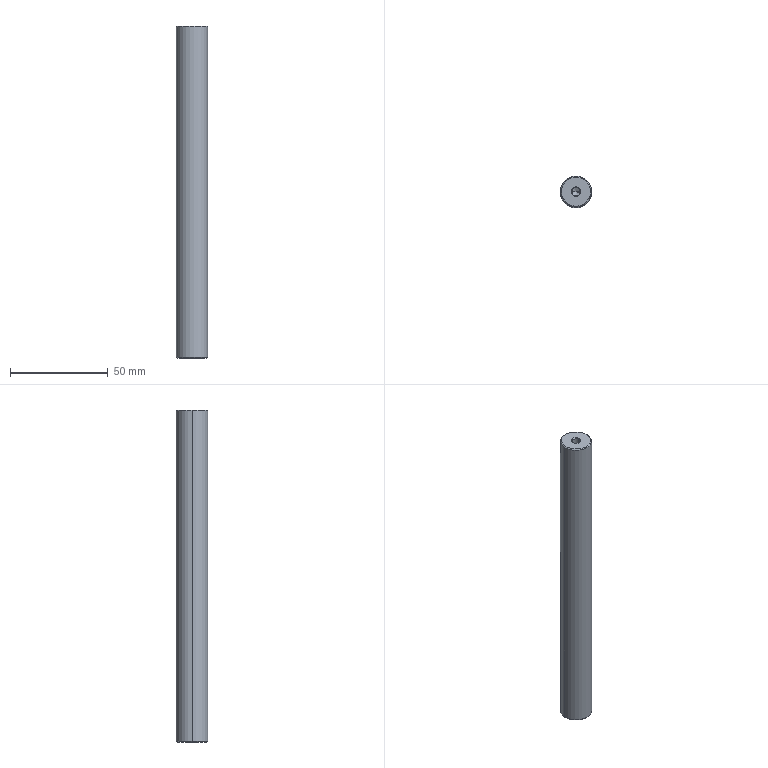Part | STEP file | 001-003-SCJ22_D16_L170_M5_N5 | 1 solid | 20 faces | box 16 x 16 x 170 mm | volume 33866 mm3 | cone 12 | cylinder 6 | plane 2 | commonest cylinder face diameters 4.134 x4 16 x2
STEP:
#1=CARTESIAN_POINT('',(0.,0.,0.));
#2=DIRECTION('',(0.,0.,1.));
#3=DIRECTION('',(1.,0.,0.));
#4=AXIS2_PLACEMENT_3D('',#1,#2,#3);
#5=CARTESIAN_POINT('',(0.,2.067,-159.25));
#6=VERTEX_POINT('',#5);
#7=CARTESIAN_POINT('',(0.,-2.067,-159.25));
#8=VERTEX_POINT('',#7);
#9=CARTESIAN_POINT('',(0.,0.,-159.25));
#10=DIRECTION('',(0.,0.,1.));
#11=DIRECTION('',(0.,-1.,0.));
#12=AXIS2_PLACEMENT_3D('',#9,#10,#11);
#13=CIRCLE('',#12,2.067);
#14=CARTESIAN_POINT('',(0.,0.,-159.25));
#15=DIRECTION('',(0.,0.,-1.));
#16=DIRECTION('',(0.,1.,0.));
#17=AXIS2_PLACEMENT_3D('',#14,#15,#16);
#18=CONICAL_SURFACE('',#17,2.067,1.047);
#19=CARTESIAN_POINT('',(9.425,0.));
#20=DIRECTION('',(-1.,0.));
#21=VECTOR('',#20,1.);
#22=LINE('',#19,#21);
#23=(GEOMETRIC_REPRESENTATION_CONTEXT(2)PARAMETRIC_REPRESENTATION_CONTEXT()REPRESENTATION_CONTEXT('',''));
#24=DEFINITIONAL_REPRESENTATION('',(#22),#23);
#25=PCURVE('',#18,#24);
#26=CARTESIAN_POINT('',(0.,0.,-170.));
#27=DIRECTION('',(0.,0.,1.));
#28=DIRECTION('',(0.,-1.,0.));
#29=AXIS2_PLACEMENT_3D('',#26,#27,#28);
#30=CYLINDRICAL_SURFACE('',#29,2.067);
#31=CARTESIAN_POINT('',(0.,10.75));
#32=DIRECTION('',(1.,0.));
#33=VECTOR('',#32,1.);
#34=LINE('',#31,#33);
#35=(GEOMETRIC_REPRESENTATION_CONTEXT(2)PARAMETRIC_REPRESENTATION_CONTEXT()REPRESENTATION_CONTEXT('',''));
#36=DEFINITIONAL_REPRESENTATION('',(#34),#35);
#37=PCURVE('',#30,#36);
#38=SURFACE_CURVE('',#13,(#25,#37),.PCURVE_S1.);
#39=EDGE_CURVE('',#6,#8,#38,.T.);
#40=ORIENTED_EDGE('',*,*,#39,.T.);
#41=CARTESIAN_POINT('',(0.,0.,-158.057));
#42=VERTEX_POINT('',#41);
#43=CARTESIAN_POINT('',(0.,-2.067,-159.25));
#44=DIRECTION('',(0.,-0.866,-0.5));
#45=VECTOR('',#44,1.);
#46=LINE('',#43,#45);
#47=CARTESIAN_POINT('',(3.142,0.));
#48=DIRECTION('',(0.,1.));
#49=VECTOR('',#48,1.);
#50=LINE('',#47,#49);
#51=(GEOMETRIC_REPRESENTATION_CONTEXT(2)PARAMETRIC_REPRESENTATION_CONTEXT()REPRESENTATION_CONTEXT('',''));
#52=DEFINITIONAL_REPRESENTATION('',(#50),#51);
#53=PCURVE('',#18,#52);
#54=CARTESIAN_POINT('',(0.,0.,-159.25));
#55=DIRECTION('',(0.,0.,-1.));
#56=DIRECTION('',(0.,1.,0.));
#57=AXIS2_PLACEMENT_3D('',#54,#55,#56);
#58=CONICAL_SURFACE('',#57,2.067,1.047);
#59=CARTESIAN_POINT('',(3.142,0.));
#60=DIRECTION('',(0.,1.));
#61=VECTOR('',#60,1.);
#62=LINE('',#59,#61);
#63=(GEOMETRIC_REPRESENTATION_CONTEXT(2)PARAMETRIC_REPRESENTATION_CONTEXT()REPRESENTATION_CONTEXT('',''));
#64=DEFINITIONAL_REPRESENTATION('',(#62),#63);
#65=PCURVE('',#58,#64);
#66=SURFACE_CURVE('',#46,(#53,#65),.PCURVE_S1.);
#67=EDGE_CURVE('',#42,#8,#66,.T.);
#68=ORIENTED_EDGE('',*,*,#67,.F.);
#69=CARTESIAN_POINT('',(0.,2.067,-159.25));
#70=DIRECTION('',(0.,0.866,-0.5));
#71=VECTOR('',#70,1.);
#72=LINE('',#69,#71);
#73=CARTESIAN_POINT('',(6.283,0.));
#74=DIRECTION('',(0.,1.));
#75=VECTOR('',#74,1.);
#76=LINE('',#73,#75);
#77=(GEOMETRIC_REPRESENTATION_CONTEXT(2)PARAMETRIC_REPRESENTATION_CONTEXT()REPRESENTATION_CONTEXT('',''));
#78=DEFINITIONAL_REPRESENTATION('',(#76),#77);
#79=PCURVE('',#18,#78);
#80=CARTESIAN_POINT('',(0.,0.));
#81=DIRECTION('',(0.,1.));
#82=VECTOR('',#81,1.);
#83=LINE('',#80,#82);
#84=(GEOMETRIC_REPRESENTATION_CONTEXT(2)PARAMETRIC_REPRESENTATION_CONTEXT()REPRESENTATION_CONTEXT('',''));
#85=DEFINITIONAL_REPRESENTATION('',(#83),#84);
#86=PCURVE('',#58,#85);
#87=SURFACE_CURVE('',#72,(#79,#86),.PCURVE_S1.);
#88=EDGE_CURVE('',#42,#6,#87,.T.);
#89=ORIENTED_EDGE('',*,*,#88,.T.);
#90=EDGE_LOOP('',(#40,#68,#89));
#91=FACE_BOUND('',#90,.F.);
#92=ADVANCED_FACE('',(#91),#18,.F.);
#93=CARTESIAN_POINT('',(0.,-2.067,-169.567));
#94=VERTEX_POINT('',#93);
#95=CARTESIAN_POINT('',(0.,-2.067,-170.));
#96=DIRECTION('',(0.,0.,1.));
#97=VECTOR('',#96,1.);
#98=LINE('',#95,#97);
#99=CARTESIAN_POINT('',(6.283,0.));
#100=DIRECTION('',(0.,1.));
#101=VECTOR('',#100,1.);
#102=LINE('',#99,#101);
#103=(GEOMETRIC_REPRESENTATION_CONTEXT(2)PARAMETRIC_REPRESENTATION_CONTEXT()REPRESENTATION_CONTEXT('',''));
#104=DEFINITIONAL_REPRESENTATION('',(#102),#103);
#105=PCURVE('',#30,#104);
#106=CARTESIAN_POINT('',(0.,0.,-170.));
#107=DIRECTION('',(0.,0.,1.));
#108=DIRECTION('',(0.,-1.,0.));
#109=AXIS2_PLACEMENT_3D('',#106,#107,#108);
#110=CYLINDRICAL_SURFACE('',#109,2.067);
#111=CARTESIAN_POINT('',(0.,0.));
#112=DIRECTION('',(0.,1.));
#113=VECTOR('',#112,1.);
#114=LINE('',#111,#113);
#115=(GEOMETRIC_REPRESENTATION_CONTEXT(2)PARAMETRIC_REPRESENTATION_CONTEXT()REPRESENTATION_CONTEXT('',''));
#116=DEFINITIONAL_REPRESENTATION('',(#114),#115);
#117=PCURVE('',#110,#116);
#118=SURFACE_CURVE('',#98,(#105,#117),.PCURVE_S1.);
#119=EDGE_CURVE('',#94,#8,#118,.T.);
#120=ORIENTED_EDGE('',*,*,#119,.T.);
#121=ORIENTED_EDGE('',*,*,#39,.F.);
#122=CARTESIAN_POINT('',(0.,2.067,-169.567));
#123=VERTEX_POINT('',#122);
#124=CARTESIAN_POINT('',(0.,2.067,-170.));
#125=DIRECTION('',(0.,0.,1.));
#126=VECTOR('',#125,1.);
#127=LINE('',#124,#126);
#128=CARTESIAN_POINT('',(3.142,0.));
#129=DIRECTION('',(0.,1.));
#130=VECTOR('',#129,1.);
#131=LINE('',#128,#130);
#132=(GEOMETRIC_REPRESENTATION_CONTEXT(2)PARAMETRIC_REPRESENTATION_CONTEXT()REPRESENTATION_CONTEXT('',''));
#133=DEFINITIONAL_REPRESENTATION('',(#131),#132);
#134=PCURVE('',#30,#133);
#135=CARTESIAN_POINT('',(3.142,0.));
#136=DIRECTION('',(0.,1.));
#137=VECTOR('',#136,1.);
#138=LINE('',#135,#137);
#139=(GEOMETRIC_REPRESENTATION_CONTEXT(2)PARAMETRIC_REPRESENTATION_CONTEXT()REPRESENTATION_CONTEXT('',''));
#140=DEFINITIONAL_REPRESENTATION('',(#138),#139);
#141=PCURVE('',#110,#140);
#142=SURFACE_CURVE('',#127,(#134,#141),.PCURVE_S1.);
#143=EDGE_CURVE('',#123,#6,#142,.T.);
#144=ORIENTED_EDGE('',*,*,#143,.F.);
#145=CARTESIAN_POINT('',(0.,0.,-169.567));
#146=DIRECTION('',(0.,0.,1.));
#147=DIRECTION('',(0.,-1.,0.));
#148=AXIS2_PLACEMENT_3D('',#145,#146,#147);
#149=CIRCLE('',#148,2.067);
#150=CARTESIAN_POINT('',(0.,0.433));
#151=DIRECTION('',(1.,0.));
#152=VECTOR('',#151,1.);
#153=LINE('',#150,#152);
#154=(GEOMETRIC_REPRESENTATION_CONTEXT(2)PARAMETRIC_REPRESENTATION_CONTEXT()REPRESENTATION_CONTEXT('',''));
#155=DEFINITIONAL_REPRESENTATION('',(#153),#154);
#156=PCURVE('',#30,#155);
#157=CARTESIAN_POINT('',(0.,0.,-170.));
#158=DIRECTION('',(0.,0.,-1.));
#159=DIRECTION('',(0.,1.,0.));
#160=AXIS2_PLACEMENT_3D('',#157,#158,#159);
#161=CONICAL_SURFACE('',#160,2.5,0.7854);
#162=CARTESIAN_POINT('',(9.425,-0.433));
#163=DIRECTION('',(-1.,0.));
#164=VECTOR('',#163,1.);
#165=LINE('',#162,#164);
#166=(GEOMETRIC_REPRESENTATION_CONTEXT(2)PARAMETRIC_REPRESENTATION_CONTEXT()REPRESENTATION_CONTEXT('',''));
#167=DEFINITIONAL_REPRESENTATION('',(#165),#166);
#168=PCURVE('',#161,#167);
#169=SURFACE_CURVE('',#149,(#156,#168),.PCURVE_S1.);
#170=EDGE_CURVE('',#123,#94,#169,.T.);
#171=ORIENTED_EDGE('',*,*,#170,.T.);
#172=EDGE_LOOP('',(#120,#121,#144,#171));
#173=FACE_BOUND('',#172,.F.);
#174=ADVANCED_FACE('',(#173),#30,.F.);
#175=CARTESIAN_POINT('',(0.,2.5,-170.));
#176=VERTEX_POINT('',#175);
#177=CARTESIAN_POINT('',(0.,2.5,-170.));
#178=DIRECTION('',(0.,0.7071,-0.7071));
#179=VECTOR('',#178,1.);
#180=LINE('',#177,#179);
#181=CARTESIAN_POINT('',(6.283,0.));
#182=DIRECTION('',(0.,1.));
#183=VECTOR('',#182,1.);
#184=LINE('',#181,#183);
#185=(GEOMETRIC_REPRESENTATION_CONTEXT(2)PARAMETRIC_REPRESENTATION_CONTEXT()REPRESENTATION_CONTEXT('',''));
#186=DEFINITIONAL_REPRESENTATION('',(#184),#185);
#187=PCURVE('',#161,#186);
#188=CARTESIAN_POINT('',(0.,0.,-170.));
#189=DIRECTION('',(0.,0.,-1.));
#190=DIRECTION('',(0.,1.,0.));
#191=AXIS2_PLACEMENT_3D('',#188,#189,#190);
#192=CONICAL_SURFACE('',#191,2.5,0.7854);
#193=CARTESIAN_POINT('',(0.,0.));
#194=DIRECTION('',(0.,1.));
#195=VECTOR('',#194,1.);
#196=LINE('',#193,#195);
#197=(GEOMETRIC_REPRESENTATION_CONTEXT(2)PARAMETRIC_REPRESENTATION_CONTEXT()REPRESENTATION_CONTEXT('',''));
#198=DEFINITIONAL_REPRESENTATION('',(#196),#197);
#199=PCURVE('',#192,#198);
#200=SURFACE_CURVE('',#180,(#187,#199),.PCURVE_S1.);
#201=EDGE_CURVE('',#123,#176,#200,.T.);
#202=ORIENTED_EDGE('',*,*,#201,.T.);
#203=CARTESIAN_POINT('',(0.,-2.5,-170.));
#204=VERTEX_POINT('',#203);
#205=CARTESIAN_POINT('',(0.,0.,-170.));
#206=DIRECTION('',(0.,0.,1.));
#207=DIRECTION('',(0.,-1.,0.));
#208=AXIS2_PLACEMENT_3D('',#205,#206,#207);
#209=CIRCLE('',#208,2.5);
#210=CARTESIAN_POINT('',(9.425,0.));
#211=DIRECTION('',(-1.,0.));
#212=VECTOR('',#211,1.);
#213=LINE('',#210,#212);
#214=(GEOMETRIC_REPRESENTATION_CONTEXT(2)PARAMETRIC_REPRESENTATION_CONTEXT()REPRESENTATION_CONTEXT('',''));
#215=DEFINITIONAL_REPRESENTATION('',(#213),#214);
#216=PCURVE('',#161,#215);
#217=CARTESIAN_POINT('',(0.,7.5,-170.));
#218=DIRECTION('',(0.,0.,1.));
#219=DIRECTION('',(1.,0.,0.));
#220=AXIS2_PLACEMENT_3D('',#217,#218,#219);
#221=PLANE('',#220);
#222=CARTESIAN_POINT('',(0.,-7.5));
#223=DIRECTION('',(0.,-1.));
#224=AXIS2_PLACEMENT_2D('',#222,#223);
#225=CIRCLE('',#224,2.5);
#226=(GEOMETRIC_REPRESENTATION_CONTEXT(2)PARAMETRIC_REPRESENTATION_CONTEXT()REPRESENTATION_CONTEXT('',''));
#227=DEFINITIONAL_REPRESENTATION('',(#225),#226);
#228=PCURVE('',#221,#227);
#229=SURFACE_CURVE('',#209,(#216,#228),.PCURVE_S1.);
#230=EDGE_CURVE('',#176,#204,#229,.T.);
#231=ORIENTED_EDGE('',*,*,#230,.T.);
#232=CARTESIAN_POINT('',(0.,-2.5,-170.));
#233=DIRECTION('',(0.,-0.7071,-0.7071));
#234=VECTOR('',#233,1.);
#235=LINE('',#232,#234);
#236=CARTESIAN_POINT('',(3.142,0.));
#237=DIRECTION('',(0.,1.));
#238=VECTOR('',#237,1.);
#239=LINE('',#236,#238);
#240=(GEOMETRIC_REPRESENTATION_CONTEXT(2)PARAMETRIC_REPRESENTATION_CONTEXT()REPRESENTATION_CONTEXT('',''));
#241=DEFINITIONAL_REPRESENTATION('',(#239),#240);
#242=PCURVE('',#161,#241);
#243=CARTESIAN_POINT('',(3.142,0.));
#244=DIRECTION('',(0.,1.));
#245=VECTOR('',#244,1.);
#246=LINE('',#243,#245);
#247=(GEOMETRIC_REPRESENTATION_CONTEXT(2)PARAMETRIC_REPRESENTATION_CONTEXT()REPRESENTATION_CONTEXT('',''));
#248=DEFINITIONAL_REPRESENTATION('',(#246),#247);
#249=PCURVE('',#192,#248);
#250=SURFACE_CURVE('',#235,(#242,#249),.PCURVE_S1.);
#251=EDGE_CURVE('',#94,#204,#250,.T.);
#252=ORIENTED_EDGE('',*,*,#251,.F.);
#253=ORIENTED_EDGE('',*,*,#170,.F.);
#254=EDGE_LOOP('',(#202,#231,#252,#253));
#255=FACE_BOUND('',#254,.F.);
#256=ADVANCED_FACE('',(#255),#161,.F.);
#257=CARTESIAN_POINT('',(-2.067,0.,-10.75));
#258=VERTEX_POINT('',#257);
#259=CARTESIAN_POINT('',(2.067,0.,-10.75));
#260=VERTEX_POINT('',#259);
#261=CARTESIAN_POINT('',(0.,0.,-10.75));
#262=DIRECTION('',(0.,0.,1.));
#263=DIRECTION('',(1.,0.,0.));
#264=AXIS2_PLACEMENT_3D('',#261,#262,#263);
#265=CIRCLE('',#264,2.067);
#266=CARTESIAN_POINT('',(0.,0.,988.057));
#267=DIRECTION('',(0.,0.,1.));
#268=DIRECTION('',(1.,0.,0.));
#269=AXIS2_PLACEMENT_3D('',#266,#267,#268);
#270=CONICAL_SURFACE('',#269,1732.051,1.047);
#271=CARTESIAN_POINT('',(0.,-998.807));
#272=DIRECTION('',(1.,0.));
#273=VECTOR('',#272,1.);
#274=LINE('',#271,#273);
#275=(GEOMETRIC_REPRESENTATION_CONTEXT(2)PARAMETRIC_REPRESENTATION_CONTEXT()REPRESENTATION_CONTEXT('',''));
#276=DEFINITIONAL_REPRESENTATION('',(#274),#275);
#277=PCURVE('',#270,#276);
#278=CARTESIAN_POINT('',(0.,0.,-11.943));
#279=DIRECTION('',(0.,0.,1.));
#280=DIRECTION('',(1.,0.,0.));
#281=AXIS2_PLACEMENT_3D('',#278,#279,#280);
#282=CYLINDRICAL_SURFACE('',#281,2.067);
#283=CARTESIAN_POINT('',(0.,1.193));
#284=DIRECTION('',(1.,0.));
#285=VECTOR('',#284,1.);
#286=LINE('',#283,#285);
#287=(GEOMETRIC_REPRESENTATION_CONTEXT(2)PARAMETRIC_REPRESENTATION_CONTEXT()REPRESENTATION_CONTEXT('',''));
#288=DEFINITIONAL_REPRESENTATION('',(#286),#287);
#289=PCURVE('',#282,#288);
#290=SURFACE_CURVE('',#265,(#277,#289),.PCURVE_S1.);
#291=EDGE_CURVE('',#258,#260,#290,.T.);
#292=ORIENTED_EDGE('',*,*,#291,.F.);
#293=CARTESIAN_POINT('',(0.,0.,-11.943));
#294=VERTEX_POINT('',#293);
#295=CARTESIAN_POINT('',(0.,0.,-11.943));
#296=DIRECTION('',(-0.866,0.,0.5));
#297=VECTOR('',#296,1.);
#298=LINE('',#295,#297);
#299=CARTESIAN_POINT('',(3.142,-1000.));
#300=CARTESIAN_POINT('',(3.142,-999.982));
#301=CARTESIAN_POINT('',(3.142,-999.946));
#302=CARTESIAN_POINT('',(3.142,-999.892));
#303=CARTESIAN_POINT('',(3.142,-999.837));
#304=CARTESIAN_POINT('',(3.142,-999.783));
#305=CARTESIAN_POINT('',(3.142,-999.729));
#306=CARTESIAN_POINT('',(3.142,-999.675));
#307=CARTESIAN_POINT('',(3.142,-999.62));
#308=CARTESIAN_POINT('',(3.142,-999.566));
#309=CARTESIAN_POINT('',(3.142,-999.512));
#310=CARTESIAN_POINT('',(3.142,-999.458));
#311=CARTESIAN_POINT('',(3.142,-999.403));
#312=CARTESIAN_POINT('',(3.142,-999.349));
#313=CARTESIAN_POINT('',(3.142,-999.295));
#314=CARTESIAN_POINT('',(3.142,-999.241));
#315=CARTESIAN_POINT('',(3.142,-999.186));
#316=CARTESIAN_POINT('',(3.142,-999.132));
#317=CARTESIAN_POINT('',(3.142,-999.078));
#318=CARTESIAN_POINT('',(3.142,-999.024));
#319=CARTESIAN_POINT('',(3.142,-998.969));
#320=CARTESIAN_POINT('',(3.142,-998.915));
#321=CARTESIAN_POINT('',(3.142,-998.861));
#322=CARTESIAN_POINT('',(3.142,-998.825));
#323=CARTESIAN_POINT('',(3.142,-998.807));
#324=B_SPLINE_CURVE_WITH_KNOTS('',3,(#299,#300,#301,#302,#303,#304,#305,#306,#307,#308,#309,#310,#311,#312,#313,#314,#315,#316,#317,#318,#319,#320,#321,#322,#323),.UNSPECIFIED.,.F.,.F.,(4,1,1,1,1,1,1,1,1,1,1,1,1,1,1,1,1,1,1,1,1,1,4),(0.,0.1085,0.217,0.3255,0.434,0.5424,0.6509,0.7594,0.8679,0.9764,1.085,1.193,1.302,1.41,1.519,1.627,1.736,1.844,1.953,2.061,2.17,2.278,2.387),.QUASI_UNIFORM_KNOTS.);
#325=(GEOMETRIC_REPRESENTATION_CONTEXT(2)PARAMETRIC_REPRESENTATION_CONTEXT()REPRESENTATION_CONTEXT('',''));
#326=DEFINITIONAL_REPRESENTATION('',(#324),#325);
#327=PCURVE('',#270,#326);
#328=CARTESIAN_POINT('',(0.,0.,988.057));
#329=DIRECTION('',(0.,0.,1.));
#330=DIRECTION('',(1.,0.,0.));
#331=AXIS2_PLACEMENT_3D('',#328,#329,#330);
#332=CONICAL_SURFACE('',#331,1732.051,1.047);
#333=CARTESIAN_POINT('',(3.142,-1000.));
#334=CARTESIAN_POINT('',(3.142,-999.982));
#335=CARTESIAN_POINT('',(3.142,-999.946));
#336=CARTESIAN_POINT('',(3.142,-999.892));
#337=CARTESIAN_POINT('',(3.142,-999.837));
#338=CARTESIAN_POINT('',(3.142,-999.783));
#339=CARTESIAN_POINT('',(3.142,-999.729));
#340=CARTESIAN_POINT('',(3.142,-999.675));
#341=CARTESIAN_POINT('',(3.142,-999.62));
#342=CARTESIAN_POINT('',(3.142,-999.566));
#343=CARTESIAN_POINT('',(3.142,-999.512));
#344=CARTESIAN_POINT('',(3.142,-999.458));
#345=CARTESIAN_POINT('',(3.142,-999.403));
#346=CARTESIAN_POINT('',(3.142,-999.349));
#347=CARTESIAN_POINT('',(3.142,-999.295));
#348=CARTESIAN_POINT('',(3.142,-999.241));
#349=CARTESIAN_POINT('',(3.142,-999.186));
#350=CARTESIAN_POINT('',(3.142,-999.132));
#351=CARTESIAN_POINT('',(3.142,-999.078));
#352=CARTESIAN_POINT('',(3.142,-999.024));
#353=CARTESIAN_POINT('',(3.142,-998.969));
#354=CARTESIAN_POINT('',(3.142,-998.915));
#355=CARTESIAN_POINT('',(3.142,-998.861));
#356=CARTESIAN_POINT('',(3.142,-998.825));
#357=CARTESIAN_POINT('',(3.142,-998.807));
#358=B_SPLINE_CURVE_WITH_KNOTS('',3,(#333,#334,#335,#336,#337,#338,#339,#340,#341,#342,#343,#344,#345,#346,#347,#348,#349,#350,#351,#352,#353,#354,#355,#356,#357),.UNSPECIFIED.,.F.,.F.,(4,1,1,1,1,1,1,1,1,1,1,1,1,1,1,1,1,1,1,1,1,1,4),(0.,0.1085,0.217,0.3255,0.434,0.5424,0.6509,0.7594,0.8679,0.9764,1.085,1.193,1.302,1.41,1.519,1.627,1.736,1.844,1.953,2.061,2.17,2.278,2.387),.QUASI_UNIFORM_KNOTS.);
#359=(GEOMETRIC_REPRESENTATION_CONTEXT(2)PARAMETRIC_REPRESENTATION_CONTEXT()REPRESENTATION_CONTEXT('',''));
#360=DEFINITIONAL_REPRESENTATION('',(#358),#359);
#361=PCURVE('',#332,#360);
#362=SURFACE_CURVE('',#298,(#327,#361),.PCURVE_S1.);
#363=EDGE_CURVE('',#294,#258,#362,.T.);
#364=ORIENTED_EDGE('',*,*,#363,.F.);
#365=CARTESIAN_POINT('',(0.,0.,-11.943));
#366=DIRECTION('',(0.866,0.,0.5));
#367=VECTOR('',#366,1.);
#368=LINE('',#365,#367);
#369=CARTESIAN_POINT('',(6.283,-1000.));
#370=DIRECTION('',(0.,1.));
#371=VECTOR('',#370,1.);
#372=LINE('',#369,#371);
#373=(GEOMETRIC_REPRESENTATION_CONTEXT(2)PARAMETRIC_REPRESENTATION_CONTEXT()REPRESENTATION_CONTEXT('',''));
#374=DEFINITIONAL_REPRESENTATION('',(#372),#373);
#375=PCURVE('',#270,#374);
#376=CARTESIAN_POINT('',(0.,-1000.));
#377=DIRECTION('',(0.,1.));
#378=VECTOR('',#377,1.);
#379=LINE('',#376,#378);
#380=(GEOMETRIC_REPRESENTATION_CONTEXT(2)PARAMETRIC_REPRESENTATION_CONTEXT()REPRESENTATION_CONTEXT('',''));
#381=DEFINITIONAL_REPRESENTATION('',(#379),#380);
#382=PCURVE('',#332,#381);
#383=SURFACE_CURVE('',#368,(#375,#382),.PCURVE_S1.);
#384=EDGE_CURVE('',#294,#260,#383,.T.);
#385=ORIENTED_EDGE('',*,*,#384,.T.);
#386=EDGE_LOOP('',(#292,#364,#385));
#387=FACE_BOUND('',#386,.F.);
#388=ADVANCED_FACE('',(#387),#270,.F.);
#389=CARTESIAN_POINT('',(2.067,0.,-0.433));
#390=VERTEX_POINT('',#389);
#391=CARTESIAN_POINT('',(2.067,0.,-11.943));
#392=DIRECTION('',(0.,0.,1.));
#393=VECTOR('',#392,1.);
#394=LINE('',#391,#393);
#395=CARTESIAN_POINT('',(6.283,0.));
#396=DIRECTION('',(0.,1.));
#397=VECTOR('',#396,1.);
#398=LINE('',#395,#397);
#399=(GEOMETRIC_REPRESENTATION_CONTEXT(2)PARAMETRIC_REPRESENTATION_CONTEXT()REPRESENTATION_CONTEXT('',''));
#400=DEFINITIONAL_REPRESENTATION('',(#398),#399);
#401=PCURVE('',#282,#400);
#402=CARTESIAN_POINT('',(0.,0.,-11.943));
#403=DIRECTION('',(0.,0.,1.));
#404=DIRECTION('',(1.,0.,0.));
#405=AXIS2_PLACEMENT_3D('',#402,#403,#404);
#406=CYLINDRICAL_SURFACE('',#405,2.067);
#407=CARTESIAN_POINT('',(0.,0.));
#408=DIRECTION('',(0.,1.));
#409=VECTOR('',#408,1.);
#410=LINE('',#407,#409);
#411=(GEOMETRIC_REPRESENTATION_CONTEXT(2)PARAMETRIC_REPRESENTATION_CONTEXT()REPRESENTATION_CONTEXT('',''));
#412=DEFINITIONAL_REPRESENTATION('',(#410),#411);
#413=PCURVE('',#406,#412);
#414=SURFACE_CURVE('',#394,(#401,#413),.PCURVE_S1.);
#415=EDGE_CURVE('',#260,#390,#414,.T.);
#416=ORIENTED_EDGE('',*,*,#415,.T.);
#417=CARTESIAN_POINT('',(-2.067,0.,-0.433));
#418=VERTEX_POINT('',#417);
#419=CARTESIAN_POINT('',(0.,0.,-0.433));
#420=DIRECTION('',(0.,0.,1.));
#421=DIRECTION('',(1.,0.,0.));
#422=AXIS2_PLACEMENT_3D('',#419,#420,#421);
#423=CIRCLE('',#422,2.067);
#424=CARTESIAN_POINT('',(0.,11.51));
#425=DIRECTION('',(1.,0.));
#426=VECTOR('',#425,1.);
#427=LINE('',#424,#426);
#428=(GEOMETRIC_REPRESENTATION_CONTEXT(2)PARAMETRIC_REPRESENTATION_CONTEXT()REPRESENTATION_CONTEXT('',''));
#429=DEFINITIONAL_REPRESENTATION('',(#427),#428);
#430=PCURVE('',#282,#429);
#431=CARTESIAN_POINT('',(0.,0.,-0.433));
#432=DIRECTION('',(0.,0.,1.));
#433=DIRECTION('',(1.,0.,0.));
#434=AXIS2_PLACEMENT_3D('',#431,#432,#433);
#435=CONICAL_SURFACE('',#434,2.067,0.7854);
#436=CARTESIAN_POINT('',(0.,0.));
#437=DIRECTION('',(1.,0.));
#438=VECTOR('',#437,1.);
#439=LINE('',#436,#438);
#440=(GEOMETRIC_REPRESENTATION_CONTEXT(2)PARAMETRIC_REPRESENTATION_CONTEXT()REPRESENTATION_CONTEXT('',''));
#441=DEFINITIONAL_REPRESENTATION('',(#439),#440);
#442=PCURVE('',#435,#441);
#443=SURFACE_CURVE('',#423,(#430,#442),.PCURVE_S1.);
#444=EDGE_CURVE('',#418,#390,#443,.T.);
#445=ORIENTED_EDGE('',*,*,#444,.F.);
#446=CARTESIAN_POINT('',(-2.067,0.,-11.943));
#447=DIRECTION('',(0.,0.,1.));
#448=VECTOR('',#447,1.);
#449=LINE('',#446,#448);
#450=CARTESIAN_POINT('',(3.142,0.));
#451=DIRECTION('',(0.,1.));
#452=VECTOR('',#451,1.);
#453=LINE('',#450,#452);
#454=(GEOMETRIC_REPRESENTATION_CONTEXT(2)PARAMETRIC_REPRESENTATION_CONTEXT()REPRESENTATION_CONTEXT('',''));
#455=DEFINITIONAL_REPRESENTATION('',(#453),#454);
#456=PCURVE('',#282,#455);
#457=CARTESIAN_POINT('',(3.142,0.));
#458=DIRECTION('',(0.,1.));
#459=VECTOR('',#458,1.);
#460=LINE('',#457,#459);
#461=(GEOMETRIC_REPRESENTATION_CONTEXT(2)PARAMETRIC_REPRESENTATION_CONTEXT()REPRESENTATION_CONTEXT('',''));
#462=DEFINITIONAL_REPRESENTATION('',(#460),#461);
#463=PCURVE('',#406,#462);
#464=SURFACE_CURVE('',#449,(#456,#463),.PCURVE_S1.);
#465=EDGE_CURVE('',#258,#418,#464,.T.);
#466=ORIENTED_EDGE('',*,*,#465,.F.);
#467=ORIENTED_EDGE('',*,*,#291,.T.);
#468=EDGE_LOOP('',(#416,#445,#466,#467));
#469=FACE_BOUND('',#468,.F.);
#470=ADVANCED_FACE('',(#469),#282,.F.);
#471=CARTESIAN_POINT('',(2.5,0.,0.));
#472=VERTEX_POINT('',#471);
#473=CARTESIAN_POINT('',(2.067,0.,-0.433));
#474=DIRECTION('',(0.7071,0.,0.7071));
#475=VECTOR('',#474,1.);
#476=LINE('',#473,#475);
#477=CARTESIAN_POINT('',(6.283,0.));
#478=DIRECTION('',(0.,1.));
#479=VECTOR('',#478,1.);
#480=LINE('',#477,#479);
#481=(GEOMETRIC_REPRESENTATION_CONTEXT(2)PARAMETRIC_REPRESENTATION_CONTEXT()REPRESENTATION_CONTEXT('',''));
#482=DEFINITIONAL_REPRESENTATION('',(#480),#481);
#483=PCURVE('',#435,#482);
#484=CARTESIAN_POINT('',(0.,0.,-0.433));
#485=DIRECTION('',(0.,0.,1.));
#486=DIRECTION('',(1.,0.,0.));
#487=AXIS2_PLACEMENT_3D('',#484,#485,#486);
#488=CONICAL_SURFACE('',#487,2.067,0.7854);
#489=CARTESIAN_POINT('',(0.,0.));
#490=DIRECTION('',(0.,1.));
#491=VECTOR('',#490,1.);
#492=LINE('',#489,#491);
#493=(GEOMETRIC_REPRESENTATION_CONTEXT(2)PARAMETRIC_REPRESENTATION_CONTEXT()REPRESENTATION_CONTEXT('',''));
#494=DEFINITIONAL_REPRESENTATION('',(#492),#493);
#495=PCURVE('',#488,#494);
#496=SURFACE_CURVE('',#476,(#483,#495),.PCURVE_S1.);
#497=EDGE_CURVE('',#390,#472,#496,.T.);
#498=ORIENTED_EDGE('',*,*,#497,.T.);
#499=CARTESIAN_POINT('',(-2.5,0.,0.));
#500=VERTEX_POINT('',#499);
#501=CARTESIAN_POINT('',(0.,0.,0.));
#502=DIRECTION('',(0.,0.,1.));
#503=DIRECTION('',(1.,0.,0.));
#504=AXIS2_PLACEMENT_3D('',#501,#502,#503);
#505=CIRCLE('',#504,2.5);
#506=CARTESIAN_POINT('',(0.,0.433));
#507=DIRECTION('',(1.,0.));
#508=VECTOR('',#507,1.);
#509=LINE('',#506,#508);
#510=(GEOMETRIC_REPRESENTATION_CONTEXT(2)PARAMETRIC_REPRESENTATION_CONTEXT()REPRESENTATION_CONTEXT('',''));
#511=DEFINITIONAL_REPRESENTATION('',(#509),#510);
#512=PCURVE('',#435,#511);
#513=CARTESIAN_POINT('',(0.,0.,0.));
#514=DIRECTION('',(0.,0.,-1.));
#515=DIRECTION('',(-1.,0.,0.));
#516=AXIS2_PLACEMENT_3D('',#513,#514,#515);
#517=PLANE('',#516);
#518=CARTESIAN_POINT('',(-2.5,0.));
#519=CARTESIAN_POINT('',(-2.5,4.33));
#520=CARTESIAN_POINT('',(1.25,2.165));
#521=CARTESIAN_POINT('',(5.,0.));
#522=CARTESIAN_POINT('',(1.25,-2.165));
#523=CARTESIAN_POINT('',(-2.5,-4.33));
#524=CARTESIAN_POINT('',(-2.5,0.));
#525=(BOUNDED_CURVE()B_SPLINE_CURVE(2,(#518,#519,#520,#521,#522,#523,#524),.UNSPECIFIED.,.T.,.F.)B_SPLINE_CURVE_WITH_KNOTS((1,2,2,2,2,1),(-2.094,0.,2.094,4.189,6.283,8.378),.UNSPECIFIED.)CURVE()GEOMETRIC_REPRESENTATION_ITEM()RATIONAL_B_SPLINE_CURVE((1.,0.5,1.,0.5,1.,0.5,1.))REPRESENTATION_ITEM(''));
#526=(GEOMETRIC_REPRESENTATION_CONTEXT(2)PARAMETRIC_REPRESENTATION_CONTEXT()REPRESENTATION_CONTEXT('',''));
#527=DEFINITIONAL_REPRESENTATION('',(#525),#526);
#528=PCURVE('',#517,#527);
#529=SURFACE_CURVE('',#505,(#512,#528),.PCURVE_S1.);
#530=EDGE_CURVE('',#500,#472,#529,.T.);
#531=ORIENTED_EDGE('',*,*,#530,.F.);
#532=CARTESIAN_POINT('',(-2.067,0.,-0.433));
#533=DIRECTION('',(-0.7071,0.,0.7071));
#534=VECTOR('',#533,1.);
#535=LINE('',#532,#534);
#536=CARTESIAN_POINT('',(3.142,0.));
#537=DIRECTION('',(0.,1.));
#538=VECTOR('',#537,1.);
#539=LINE('',#536,#538);
#540=(GEOMETRIC_REPRESENTATION_CONTEXT(2)PARAMETRIC_REPRESENTATION_CONTEXT()REPRESENTATION_CONTEXT('',''));
#541=DEFINITIONAL_REPRESENTATION('',(#539),#540);
#542=PCURVE('',#435,#541);
#543=CARTESIAN_POINT('',(3.142,0.));
#544=DIRECTION('',(0.,1.));
#545=VECTOR('',#544,1.);
#546=LINE('',#543,#545);
#547=(GEOMETRIC_REPRESENTATION_CONTEXT(2)PARAMETRIC_REPRESENTATION_CONTEXT()REPRESENTATION_CONTEXT('',''));
#548=DEFINITIONAL_REPRESENTATION('',(#546),#547);
#549=PCURVE('',#488,#548);
#550=SURFACE_CURVE('',#535,(#542,#549),.PCURVE_S1.);
#551=EDGE_CURVE('',#418,#500,#550,.T.);
#552=ORIENTED_EDGE('',*,*,#551,.F.);
#553=ORIENTED_EDGE('',*,*,#444,.T.);
#554=EDGE_LOOP('',(#498,#531,#552,#553));
#555=FACE_BOUND('',#554,.F.);
#556=ADVANCED_FACE('',(#555),#435,.F.);
#557=CARTESIAN_POINT('',(7.5,0.,-170.));
#558=VERTEX_POINT('',#557);
#559=CARTESIAN_POINT('',(-7.5,0.,-170.));
#560=VERTEX_POINT('',#559);
#561=CARTESIAN_POINT('',(0.,0.,-170.));
#562=DIRECTION('',(0.,0.,1.));
#563=DIRECTION('',(1.,0.,0.));
#564=AXIS2_PLACEMENT_3D('',#561,#562,#563);
#565=CIRCLE('',#564,7.5);
#566=CARTESIAN_POINT('',(0.,0.,-170.));
#567=DIRECTION('',(0.,0.,1.));
#568=DIRECTION('',(1.,0.,0.));
#569=AXIS2_PLACEMENT_3D('',#566,#567,#568);
#570=CONICAL_SURFACE('',#569,7.5,0.7854);
#571=CARTESIAN_POINT('',(0.,0.));
#572=DIRECTION('',(1.,0.));
#573=VECTOR('',#572,1.);
#574=LINE('',#571,#573);
#575=(GEOMETRIC_REPRESENTATION_CONTEXT(2)PARAMETRIC_REPRESENTATION_CONTEXT()REPRESENTATION_CONTEXT('',''));
#576=DEFINITIONAL_REPRESENTATION('',(#574),#575);
#577=PCURVE('',#570,#576);
#578=CARTESIAN_POINT('',(0.,-7.5));
#579=DIRECTION('',(1.,0.));
#580=AXIS2_PLACEMENT_2D('',#578,#579);
#581=CIRCLE('',#580,7.5);
#582=(GEOMETRIC_REPRESENTATION_CONTEXT(2)PARAMETRIC_REPRESENTATION_CONTEXT()REPRESENTATION_CONTEXT('',''));
#583=DEFINITIONAL_REPRESENTATION('',(#581),#582);
#584=PCURVE('',#221,#583);
#585=SURFACE_CURVE('',#565,(#577,#584),.PCURVE_S1.);
#586=EDGE_CURVE('',#558,#560,#585,.T.);
#587=ORIENTED_EDGE('',*,*,#586,.T.);
#588=CARTESIAN_POINT('',(-8.,0.,-169.5));
#589=VERTEX_POINT('',#588);
#590=CARTESIAN_POINT('',(-7.5,0.,-170.));
#591=DIRECTION('',(-0.7071,0.,0.7071));
#592=VECTOR('',#591,1.);
#593=LINE('',#590,#592);
#594=CARTESIAN_POINT('',(3.142,0.));
#595=DIRECTION('',(0.,1.));
#596=VECTOR('',#595,1.);
#597=LINE('',#594,#596);
#598=(GEOMETRIC_REPRESENTATION_CONTEXT(2)PARAMETRIC_REPRESENTATION_CONTEXT()REPRESENTATION_CONTEXT('',''));
#599=DEFINITIONAL_REPRESENTATION('',(#597),#598);
#600=PCURVE('',#570,#599);
#601=CARTESIAN_POINT('',(0.,0.,-170.));
#602=DIRECTION('',(0.,0.,1.));
#603=DIRECTION('',(1.,0.,0.));
#604=AXIS2_PLACEMENT_3D('',#601,#602,#603);
#605=CONICAL_SURFACE('',#604,7.5,0.7854);
#606=CARTESIAN_POINT('',(3.142,0.));
#607=DIRECTION('',(0.,1.));
#608=VECTOR('',#607,1.);
#609=LINE('',#606,#608);
#610=(GEOMETRIC_REPRESENTATION_CONTEXT(2)PARAMETRIC_REPRESENTATION_CONTEXT()REPRESENTATION_CONTEXT('',''));
#611=DEFINITIONAL_REPRESENTATION('',(#609),#610);
#612=PCURVE('',#605,#611);
#613=SURFACE_CURVE('',#593,(#600,#612),.PCURVE_S1.);
#614=EDGE_CURVE('',#560,#589,#613,.T.);
#615=ORIENTED_EDGE('',*,*,#614,.T.);
#616=CARTESIAN_POINT('',(8.,0.,-169.5));
#617=VERTEX_POINT('',#616);
#618=CARTESIAN_POINT('',(0.,0.,-169.5));
#619=DIRECTION('',(0.,0.,1.));
#620=DIRECTION('',(1.,0.,0.));
#621=AXIS2_PLACEMENT_3D('',#618,#619,#620);
#622=CIRCLE('',#621,8.);
#623=CARTESIAN_POINT('',(0.,0.5));
#624=DIRECTION('',(1.,0.));
#625=VECTOR('',#624,1.);
#626=LINE('',#623,#625);
#627=(GEOMETRIC_REPRESENTATION_CONTEXT(2)PARAMETRIC_REPRESENTATION_CONTEXT()REPRESENTATION_CONTEXT('',''));
#628=DEFINITIONAL_REPRESENTATION('',(#626),#627);
#629=PCURVE('',#570,#628);
#630=CARTESIAN_POINT('',(0.,0.,-170.));
#631=DIRECTION('',(0.,0.,1.));
#632=DIRECTION('',(1.,0.,0.));
#633=AXIS2_PLACEMENT_3D('',#630,#631,#632);
#634=CYLINDRICAL_SURFACE('',#633,8.);
#635=CARTESIAN_POINT('',(0.,0.5));
#636=DIRECTION('',(1.,0.));
#637=VECTOR('',#636,1.);
#638=LINE('',#635,#637);
#639=(GEOMETRIC_REPRESENTATION_CONTEXT(2)PARAMETRIC_REPRESENTATION_CONTEXT()REPRESENTATION_CONTEXT('',''));
#640=DEFINITIONAL_REPRESENTATION('',(#638),#639);
#641=PCURVE('',#634,#640);
#642=SURFACE_CURVE('',#622,(#629,#641),.PCURVE_S1.);
#643=EDGE_CURVE('',#617,#589,#642,.T.);
#644=ORIENTED_EDGE('',*,*,#643,.F.);
#645=CARTESIAN_POINT('',(7.5,0.,-170.));
#646=DIRECTION('',(0.7071,0.,0.7071));
#647=VECTOR('',#646,1.);
#648=LINE('',#645,#647);
#649=CARTESIAN_POINT('',(0.,0.));
#650=DIRECTION('',(0.,1.));
#651=VECTOR('',#650,1.);
#652=LINE('',#649,#651);
#653=(GEOMETRIC_REPRESENTATION_CONTEXT(2)PARAMETRIC_REPRESENTATION_CONTEXT()REPRESENTATION_CONTEXT('',''));
#654=DEFINITIONAL_REPRESENTATION('',(#652),#653);
#655=PCURVE('',#570,#654);
#656=CARTESIAN_POINT('',(6.283,0.));
#657=DIRECTION('',(0.,1.));
#658=VECTOR('',#657,1.);
#659=LINE('',#656,#658);
#660=(GEOMETRIC_REPRESENTATION_CONTEXT(2)PARAMETRIC_REPRESENTATION_CONTEXT()REPRESENTATION_CONTEXT('',''));
#661=DEFINITIONAL_REPRESENTATION('',(#659),#660);
#662=PCURVE('',#605,#661);
#663=SURFACE_CURVE('',#648,(#655,#662),.PCURVE_S1.);
#664=EDGE_CURVE('',#558,#617,#663,.T.);
#665=ORIENTED_EDGE('',*,*,#664,.F.);
#666=EDGE_LOOP('',(#587,#615,#644,#665));
#667=FACE_BOUND('',#666,.T.);
#668=ADVANCED_FACE('',(#667),#570,.T.);
#669=ORIENTED_EDGE('',*,*,#643,.T.);
#670=CARTESIAN_POINT('',(-8.,0.,-0.5));
#671=VERTEX_POINT('',#670);
#672=CARTESIAN_POINT('',(-8.,0.,-170.));
#673=DIRECTION('',(0.,0.,1.));
#674=VECTOR('',#673,1.);
#675=LINE('',#672,#674);
#676=CARTESIAN_POINT('',(3.142,0.));
#677=DIRECTION('',(0.,1.));
#678=VECTOR('',#677,1.);
#679=LINE('',#676,#678);
#680=(GEOMETRIC_REPRESENTATION_CONTEXT(2)PARAMETRIC_REPRESENTATION_CONTEXT()REPRESENTATION_CONTEXT('',''));
#681=DEFINITIONAL_REPRESENTATION('',(#679),#680);
#682=PCURVE('',#634,#681);
#683=CARTESIAN_POINT('',(0.,0.,-170.));
#684=DIRECTION('',(0.,0.,1.));
#685=DIRECTION('',(1.,0.,0.));
#686=AXIS2_PLACEMENT_3D('',#683,#684,#685);
#687=CYLINDRICAL_SURFACE('',#686,8.);
#688=CARTESIAN_POINT('',(3.142,0.));
#689=DIRECTION('',(0.,1.));
#690=VECTOR('',#689,1.);
#691=LINE('',#688,#690);
#692=(GEOMETRIC_REPRESENTATION_CONTEXT(2)PARAMETRIC_REPRESENTATION_CONTEXT()REPRESENTATION_CONTEXT('',''));
#693=DEFINITIONAL_REPRESENTATION('',(#691),#692);
#694=PCURVE('',#687,#693);
#695=SURFACE_CURVE('',#675,(#682,#694),.PCURVE_S1.);
#696=EDGE_CURVE('',#589,#671,#695,.T.);
#697=ORIENTED_EDGE('',*,*,#696,.T.);
#698=CARTESIAN_POINT('',(8.,0.,-0.5));
#699=VERTEX_POINT('',#698);
#700=CARTESIAN_POINT('',(0.,0.,-0.5));
#701=DIRECTION('',(0.,0.,1.));
#702=DIRECTION('',(1.,0.,0.));
#703=AXIS2_PLACEMENT_3D('',#700,#701,#702);
#704=CIRCLE('',#703,8.);
#705=CARTESIAN_POINT('',(0.,169.5));
#706=DIRECTION('',(1.,0.));
#707=VECTOR('',#706,1.);
#708=LINE('',#705,#707);
#709=(GEOMETRIC_REPRESENTATION_CONTEXT(2)PARAMETRIC_REPRESENTATION_CONTEXT()REPRESENTATION_CONTEXT('',''));
#710=DEFINITIONAL_REPRESENTATION('',(#708),#709);
#711=PCURVE('',#634,#710);
#712=CARTESIAN_POINT('',(0.,0.,-0.5));
#713=DIRECTION('',(0.,0.,-1.));
#714=DIRECTION('',(-1.,0.,0.));
#715=AXIS2_PLACEMENT_3D('',#712,#713,#714);
#716=CONICAL_SURFACE('',#715,8.,0.7854);
#717=CARTESIAN_POINT('',(3.142,0.));
#718=DIRECTION('',(-1.,0.));
#719=VECTOR('',#718,1.);
#720=LINE('',#717,#719);
#721=(GEOMETRIC_REPRESENTATION_CONTEXT(2)PARAMETRIC_REPRESENTATION_CONTEXT()REPRESENTATION_CONTEXT('',''));
#722=DEFINITIONAL_REPRESENTATION('',(#720),#721);
#723=PCURVE('',#716,#722);
#724=SURFACE_CURVE('',#704,(#711,#723),.PCURVE_S1.);
#725=EDGE_CURVE('',#699,#671,#724,.T.);
#726=ORIENTED_EDGE('',*,*,#725,.F.);
#727=CARTESIAN_POINT('',(8.,0.,-170.));
#728=DIRECTION('',(0.,0.,1.));
#729=VECTOR('',#728,1.);
#730=LINE('',#727,#729);
#731=CARTESIAN_POINT('',(0.,0.));
#732=DIRECTION('',(0.,1.));
#733=VECTOR('',#732,1.);
#734=LINE('',#731,#733);
#735=(GEOMETRIC_REPRESENTATION_CONTEXT(2)PARAMETRIC_REPRESENTATION_CONTEXT()REPRESENTATION_CONTEXT('',''));
#736=DEFINITIONAL_REPRESENTATION('',(#734),#735);
#737=PCURVE('',#634,#736);
#738=CARTESIAN_POINT('',(6.283,0.));
#739=DIRECTION('',(0.,1.));
#740=VECTOR('',#739,1.);
#741=LINE('',#738,#740);
#742=(GEOMETRIC_REPRESENTATION_CONTEXT(2)PARAMETRIC_REPRESENTATION_CONTEXT()REPRESENTATION_CONTEXT('',''));
#743=DEFINITIONAL_REPRESENTATION('',(#741),#742);
#744=PCURVE('',#687,#743);
#745=SURFACE_CURVE('',#730,(#737,#744),.PCURVE_S1.);
#746=EDGE_CURVE('',#617,#699,#745,.T.);
#747=ORIENTED_EDGE('',*,*,#746,.F.);
#748=EDGE_LOOP('',(#669,#697,#726,#747));
#749=FACE_BOUND('',#748,.T.);
#750=ADVANCED_FACE('',(#749),#634,.T.);
#751=CARTESIAN_POINT('',(7.5,0.,0.));
#752=VERTEX_POINT('',#751);
#753=CARTESIAN_POINT('',(-7.5,0.,0.));
#754=VERTEX_POINT('',#753);
#755=CARTESIAN_POINT('',(0.,0.,0.));
#756=DIRECTION('',(0.,0.,1.));
#757=DIRECTION('',(1.,0.,0.));
#758=AXIS2_PLACEMENT_3D('',#755,#756,#757);
#759=CIRCLE('',#758,7.5);
#760=CARTESIAN_POINT('',(3.142,-0.5));
#761=DIRECTION('',(-1.,0.));
#762=VECTOR('',#761,1.);
#763=LINE('',#760,#762);
#764=(GEOMETRIC_REPRESENTATION_CONTEXT(2)PARAMETRIC_REPRESENTATION_CONTEXT()REPRESENTATION_CONTEXT('',''));
#765=DEFINITIONAL_REPRESENTATION('',(#763),#764);
#766=PCURVE('',#716,#765);
#767=CARTESIAN_POINT('',(-7.5,0.));
#768=CARTESIAN_POINT('',(-7.5,12.99));
#769=CARTESIAN_POINT('',(3.75,6.495));
#770=CARTESIAN_POINT('',(15.,0.));
#771=CARTESIAN_POINT('',(3.75,-6.495));
#772=CARTESIAN_POINT('',(-7.5,-12.99));
#773=CARTESIAN_POINT('',(-7.5,0.));
#774=(BOUNDED_CURVE()B_SPLINE_CURVE(2,(#767,#768,#769,#770,#771,#772,#773),.UNSPECIFIED.,.T.,.F.)B_SPLINE_CURVE_WITH_KNOTS((1,2,2,2,2,1),(-2.094,0.,2.094,4.189,6.283,8.378),.UNSPECIFIED.)CURVE()GEOMETRIC_REPRESENTATION_ITEM()RATIONAL_B_SPLINE_CURVE((1.,0.5,1.,0.5,1.,0.5,1.))REPRESENTATION_ITEM(''));
#775=(GEOMETRIC_REPRESENTATION_CONTEXT(2)PARAMETRIC_REPRESENTATION_CONTEXT()REPRESENTATION_CONTEXT('',''));
#776=DEFINITIONAL_REPRESENTATION('',(#774),#775);
#777=PCURVE('',#517,#776);
#778=SURFACE_CURVE('',#759,(#766,#777),.PCURVE_S1.);
#779=EDGE_CURVE('',#752,#754,#778,.T.);
#780=ORIENTED_EDGE('',*,*,#779,.F.);
#781=CARTESIAN_POINT('',(8.,0.,-0.5));
#782=DIRECTION('',(0.7071,0.,-0.7071));
#783=VECTOR('',#782,1.);
#784=LINE('',#781,#783);
#785=CARTESIAN_POINT('',(3.142,0.));
#786=DIRECTION('',(0.,1.));
#787=VECTOR('',#786,1.);
#788=LINE('',#785,#787);
#789=(GEOMETRIC_REPRESENTATION_CONTEXT(2)PARAMETRIC_REPRESENTATION_CONTEXT()REPRESENTATION_CONTEXT('',''));
#790=DEFINITIONAL_REPRESENTATION('',(#788),#789);
#791=PCURVE('',#716,#790);
#792=CARTESIAN_POINT('',(0.,0.,-0.5));
#793=DIRECTION('',(0.,0.,-1.));
#794=DIRECTION('',(-1.,0.,0.));
#795=AXIS2_PLACEMENT_3D('',#792,#793,#794);
#796=CONICAL_SURFACE('',#795,8.,0.7854);
#797=CARTESIAN_POINT('',(3.142,0.));
#798=DIRECTION('',(0.,1.));
#799=VECTOR('',#798,1.);
#800=LINE('',#797,#799);
#801=(GEOMETRIC_REPRESENTATION_CONTEXT(2)PARAMETRIC_REPRESENTATION_CONTEXT()REPRESENTATION_CONTEXT('',''));
#802=DEFINITIONAL_REPRESENTATION('',(#800),#801);
#803=PCURVE('',#796,#802);
#804=SURFACE_CURVE('',#784,(#791,#803),.PCURVE_S1.);
#805=EDGE_CURVE('',#752,#699,#804,.T.);
#806=ORIENTED_EDGE('',*,*,#805,.T.);
#807=ORIENTED_EDGE('',*,*,#725,.T.);
#808=CARTESIAN_POINT('',(-8.,0.,-0.5));
#809=DIRECTION('',(-0.7071,0.,-0.7071));
#810=VECTOR('',#809,1.);
#811=LINE('',#808,#810);
#812=CARTESIAN_POINT('',(0.,0.));
#813=DIRECTION('',(0.,1.));
#814=VECTOR('',#813,1.);
#815=LINE('',#812,#814);
#816=(GEOMETRIC_REPRESENTATION_CONTEXT(2)PARAMETRIC_REPRESENTATION_CONTEXT()REPRESENTATION_CONTEXT('',''));
#817=DEFINITIONAL_REPRESENTATION('',(#815),#816);
#818=PCURVE('',#716,#817);
#819=CARTESIAN_POINT('',(6.283,0.));
#820=DIRECTION('',(0.,1.));
#821=VECTOR('',#820,1.);
#822=LINE('',#819,#821);
#823=(GEOMETRIC_REPRESENTATION_CONTEXT(2)PARAMETRIC_REPRESENTATION_CONTEXT()REPRESENTATION_CONTEXT('',''));
#824=DEFINITIONAL_REPRESENTATION('',(#822),#823);
#825=PCURVE('',#796,#824);
#826=SURFACE_CURVE('',#811,(#818,#825),.PCURVE_S1.);
#827=EDGE_CURVE('',#754,#671,#826,.T.);
#828=ORIENTED_EDGE('',*,*,#827,.F.);
#829=EDGE_LOOP('',(#780,#806,#807,#828));
#830=FACE_BOUND('',#829,.T.);
#831=ADVANCED_FACE('',(#830),#716,.T.);
#832=CARTESIAN_POINT('',(0.,0.,0.));
#833=DIRECTION('',(0.,0.,1.));
#834=DIRECTION('',(1.,0.,0.));
#835=AXIS2_PLACEMENT_3D('',#832,#833,#834);
#836=CIRCLE('',#835,2.5);
#837=CARTESIAN_POINT('',(-2.5,0.));
#838=CARTESIAN_POINT('',(-2.5,4.33));
#839=CARTESIAN_POINT('',(1.25,2.165));
#840=CARTESIAN_POINT('',(5.,0.));
#841=CARTESIAN_POINT('',(1.25,-2.165));
#842=CARTESIAN_POINT('',(-2.5,-4.33));
#843=CARTESIAN_POINT('',(-2.5,0.));
#844=(BOUNDED_CURVE()B_SPLINE_CURVE(2,(#837,#838,#839,#840,#841,#842,#843),.UNSPECIFIED.,.T.,.F.)B_SPLINE_CURVE_WITH_KNOTS((1,2,2,2,2,1),(-2.094,0.,2.094,4.189,6.283,8.378),.UNSPECIFIED.)CURVE()GEOMETRIC_REPRESENTATION_ITEM()RATIONAL_B_SPLINE_CURVE((1.,0.5,1.,0.5,1.,0.5,1.))REPRESENTATION_ITEM(''));
#845=(GEOMETRIC_REPRESENTATION_CONTEXT(2)PARAMETRIC_REPRESENTATION_CONTEXT()REPRESENTATION_CONTEXT('',''));
#846=DEFINITIONAL_REPRESENTATION('',(#844),#845);
#847=PCURVE('',#517,#846);
#848=CARTESIAN_POINT('',(0.,0.433));
#849=DIRECTION('',(1.,0.));
#850=VECTOR('',#849,1.);
#851=LINE('',#848,#850);
#852=(GEOMETRIC_REPRESENTATION_CONTEXT(2)PARAMETRIC_REPRESENTATION_CONTEXT()REPRESENTATION_CONTEXT('',''));
#853=DEFINITIONAL_REPRESENTATION('',(#851),#852);
#854=PCURVE('',#488,#853);
#855=SURFACE_CURVE('',#836,(#847,#854),.PCURVE_S1.);
#856=EDGE_CURVE('',#472,#500,#855,.T.);
#857=ORIENTED_EDGE('',*,*,#856,.F.);
#858=ORIENTED_EDGE('',*,*,#530,.F.);
#859=EDGE_LOOP('',(#857,#858));
#860=FACE_BOUND('',#859,.T.);
#861=CARTESIAN_POINT('',(0.,0.,0.));
#862=DIRECTION('',(0.,0.,1.));
#863=DIRECTION('',(1.,0.,0.));
#864=AXIS2_PLACEMENT_3D('',#861,#862,#863);
#865=CIRCLE('',#864,7.5);
#866=CARTESIAN_POINT('',(-7.5,0.));
#867=CARTESIAN_POINT('',(-7.5,12.99));
#868=CARTESIAN_POINT('',(3.75,6.495));
#869=CARTESIAN_POINT('',(15.,0.));
#870=CARTESIAN_POINT('',(3.75,-6.495));
#871=CARTESIAN_POINT('',(-7.5,-12.99));
#872=CARTESIAN_POINT('',(-7.5,0.));
#873=(BOUNDED_CURVE()B_SPLINE_CURVE(2,(#866,#867,#868,#869,#870,#871,#872),.UNSPECIFIED.,.T.,.F.)B_SPLINE_CURVE_WITH_KNOTS((1,2,2,2,2,1),(-2.094,0.,2.094,4.189,6.283,8.378),.UNSPECIFIED.)CURVE()GEOMETRIC_REPRESENTATION_ITEM()RATIONAL_B_SPLINE_CURVE((1.,0.5,1.,0.5,1.,0.5,1.))REPRESENTATION_ITEM(''));
#874=(GEOMETRIC_REPRESENTATION_CONTEXT(2)PARAMETRIC_REPRESENTATION_CONTEXT()REPRESENTATION_CONTEXT('',''));
#875=DEFINITIONAL_REPRESENTATION('',(#873),#874);
#876=PCURVE('',#517,#875);
#877=CARTESIAN_POINT('',(9.425,-0.5));
#878=DIRECTION('',(-1.,0.));
#879=VECTOR('',#878,1.);
#880=LINE('',#877,#879);
#881=(GEOMETRIC_REPRESENTATION_CONTEXT(2)PARAMETRIC_REPRESENTATION_CONTEXT()REPRESENTATION_CONTEXT('',''));
#882=DEFINITIONAL_REPRESENTATION('',(#880),#881);
#883=PCURVE('',#796,#882);
#884=SURFACE_CURVE('',#865,(#876,#883),.PCURVE_S1.);
#885=EDGE_CURVE('',#754,#752,#884,.T.);
#886=ORIENTED_EDGE('',*,*,#885,.T.);
#887=ORIENTED_EDGE('',*,*,#779,.T.);
#888=EDGE_LOOP('',(#886,#887));
#889=FACE_BOUND('',#888,.T.);
#890=ADVANCED_FACE('',(#860,#889),#517,.F.);
#891=ORIENTED_EDGE('',*,*,#805,.F.);
#892=ORIENTED_EDGE('',*,*,#885,.F.);
#893=ORIENTED_EDGE('',*,*,#827,.T.);
#894=CARTESIAN_POINT('',(0.,0.,-0.5));
#895=DIRECTION('',(0.,0.,1.));
#896=DIRECTION('',(1.,0.,0.));
#897=AXIS2_PLACEMENT_3D('',#894,#895,#896);
#898=CIRCLE('',#897,8.);
#899=CARTESIAN_POINT('',(9.425,0.));
#900=DIRECTION('',(-1.,0.));
#901=VECTOR('',#900,1.);
#902=LINE('',#899,#901);
#903=(GEOMETRIC_REPRESENTATION_CONTEXT(2)PARAMETRIC_REPRESENTATION_CONTEXT()REPRESENTATION_CONTEXT('',''));
#904=DEFINITIONAL_REPRESENTATION('',(#902),#903);
#905=PCURVE('',#796,#904);
#906=CARTESIAN_POINT('',(0.,169.5));
#907=DIRECTION('',(1.,0.));
#908=VECTOR('',#907,1.);
#909=LINE('',#906,#908);
#910=(GEOMETRIC_REPRESENTATION_CONTEXT(2)PARAMETRIC_REPRESENTATION_CONTEXT()REPRESENTATION_CONTEXT('',''));
#911=DEFINITIONAL_REPRESENTATION('',(#909),#910);
#912=PCURVE('',#687,#911);
#913=SURFACE_CURVE('',#898,(#905,#912),.PCURVE_S1.);
#914=EDGE_CURVE('',#671,#699,#913,.T.);
#915=ORIENTED_EDGE('',*,*,#914,.T.);
#916=EDGE_LOOP('',(#891,#892,#893,#915));
#917=FACE_BOUND('',#916,.T.);
#918=ADVANCED_FACE('',(#917),#796,.T.);
#919=ORIENTED_EDGE('',*,*,#696,.F.);
#920=CARTESIAN_POINT('',(0.,0.,-169.5));
#921=DIRECTION('',(0.,0.,1.));
#922=DIRECTION('',(1.,0.,0.));
#923=AXIS2_PLACEMENT_3D('',#920,#921,#922);
#924=CIRCLE('',#923,8.);
#925=CARTESIAN_POINT('',(0.,0.5));
#926=DIRECTION('',(1.,0.));
#927=VECTOR('',#926,1.);
#928=LINE('',#925,#927);
#929=(GEOMETRIC_REPRESENTATION_CONTEXT(2)PARAMETRIC_REPRESENTATION_CONTEXT()REPRESENTATION_CONTEXT('',''));
#930=DEFINITIONAL_REPRESENTATION('',(#928),#929);
#931=PCURVE('',#687,#930);
#932=CARTESIAN_POINT('',(0.,0.5));
#933=DIRECTION('',(1.,0.));
#934=VECTOR('',#933,1.);
#935=LINE('',#932,#934);
#936=(GEOMETRIC_REPRESENTATION_CONTEXT(2)PARAMETRIC_REPRESENTATION_CONTEXT()REPRESENTATION_CONTEXT('',''));
#937=DEFINITIONAL_REPRESENTATION('',(#935),#936);
#938=PCURVE('',#605,#937);
#939=SURFACE_CURVE('',#924,(#931,#938),.PCURVE_S1.);
#940=EDGE_CURVE('',#589,#617,#939,.T.);
#941=ORIENTED_EDGE('',*,*,#940,.T.);
#942=ORIENTED_EDGE('',*,*,#746,.T.);
#943=ORIENTED_EDGE('',*,*,#914,.F.);
#944=EDGE_LOOP('',(#919,#941,#942,#943));
#945=FACE_BOUND('',#944,.T.);
#946=ADVANCED_FACE('',(#945),#687,.T.);
#947=ORIENTED_EDGE('',*,*,#614,.F.);
#948=CARTESIAN_POINT('',(0.,0.,-170.));
#949=DIRECTION('',(0.,0.,1.));
#950=DIRECTION('',(1.,0.,0.));
#951=AXIS2_PLACEMENT_3D('',#948,#949,#950);
#952=CIRCLE('',#951,7.5);
#953=CARTESIAN_POINT('',(0.,0.));
#954=DIRECTION('',(1.,0.));
#955=VECTOR('',#954,1.);
#956=LINE('',#953,#955);
#957=(GEOMETRIC_REPRESENTATION_CONTEXT(2)PARAMETRIC_REPRESENTATION_CONTEXT()REPRESENTATION_CONTEXT('',''));
#958=DEFINITIONAL_REPRESENTATION('',(#956),#957);
#959=PCURVE('',#605,#958);
#960=CARTESIAN_POINT('',(0.,-7.5));
#961=DIRECTION('',(1.,0.));
#962=AXIS2_PLACEMENT_2D('',#960,#961);
#963=CIRCLE('',#962,7.5);
#964=(GEOMETRIC_REPRESENTATION_CONTEXT(2)PARAMETRIC_REPRESENTATION_CONTEXT()REPRESENTATION_CONTEXT('',''));
#965=DEFINITIONAL_REPRESENTATION('',(#963),#964);
#966=PCURVE('',#221,#965);
#967=SURFACE_CURVE('',#952,(#959,#966),.PCURVE_S1.);
#968=EDGE_CURVE('',#560,#558,#967,.T.);
#969=ORIENTED_EDGE('',*,*,#968,.T.);
#970=ORIENTED_EDGE('',*,*,#664,.T.);
#971=ORIENTED_EDGE('',*,*,#940,.F.);
#972=EDGE_LOOP('',(#947,#969,#970,#971));
#973=FACE_BOUND('',#972,.T.);
#974=ADVANCED_FACE('',(#973),#605,.T.);
#975=ORIENTED_EDGE('',*,*,#230,.T.);
#976=CARTESIAN_POINT('',(0.,0.,-170.));
#977=DIRECTION('',(0.,0.,1.));
#978=DIRECTION('',(0.,-1.,0.));
#979=AXIS2_PLACEMENT_3D('',#976,#977,#978);
#980=CIRCLE('',#979,2.5);
#981=CARTESIAN_POINT('',(0.,-7.5));
#982=DIRECTION('',(0.,-1.));
#983=AXIS2_PLACEMENT_2D('',#981,#982);
#984=CIRCLE('',#983,2.5);
#985=(GEOMETRIC_REPRESENTATION_CONTEXT(2)PARAMETRIC_REPRESENTATION_CONTEXT()REPRESENTATION_CONTEXT('',''));
#986=DEFINITIONAL_REPRESENTATION('',(#984),#985);
#987=PCURVE('',#221,#986);
#988=CARTESIAN_POINT('',(3.142,0.));
#989=DIRECTION('',(-1.,0.));
#990=VECTOR('',#989,1.);
#991=LINE('',#988,#990);
#992=(GEOMETRIC_REPRESENTATION_CONTEXT(2)PARAMETRIC_REPRESENTATION_CONTEXT()REPRESENTATION_CONTEXT('',''));
#993=DEFINITIONAL_REPRESENTATION('',(#991),#992);
#994=PCURVE('',#192,#993);
#995=SURFACE_CURVE('',#980,(#987,#994),.PCURVE_S1.);
#996=EDGE_CURVE('',#204,#176,#995,.T.);
#997=ORIENTED_EDGE('',*,*,#996,.T.);
#998=EDGE_LOOP('',(#975,#997));
#999=FACE_BOUND('',#998,.T.);
#1000=ORIENTED_EDGE('',*,*,#586,.F.);
#1001=ORIENTED_EDGE('',*,*,#968,.F.);
#1002=EDGE_LOOP('',(#1000,#1001));
#1003=FACE_BOUND('',#1002,.T.);
#1004=ADVANCED_FACE('',(#999,#1003),#221,.F.);
#1005=ORIENTED_EDGE('',*,*,#856,.F.);
#1006=ORIENTED_EDGE('',*,*,#497,.F.);
#1007=CARTESIAN_POINT('',(0.,0.,-0.433));
#1008=DIRECTION('',(0.,0.,1.));
#1009=DIRECTION('',(1.,0.,0.));
#1010=AXIS2_PLACEMENT_3D('',#1007,#1008,#1009);
#1011=CIRCLE('',#1010,2.067);
#1012=CARTESIAN_POINT('',(0.,0.));
#1013=DIRECTION('',(1.,0.));
#1014=VECTOR('',#1013,1.);
#1015=LINE('',#1012,#1014);
#1016=(GEOMETRIC_REPRESENTATION_CONTEXT(2)PARAMETRIC_REPRESENTATION_CONTEXT()REPRESENTATION_CONTEXT('',''));
#1017=DEFINITIONAL_REPRESENTATION('',(#1015),#1016);
#1018=PCURVE('',#488,#1017);
#1019=CARTESIAN_POINT('',(0.,11.51));
#1020=DIRECTION('',(1.,0.));
#1021=VECTOR('',#1020,1.);
#1022=LINE('',#1019,#1021);
#1023=(GEOMETRIC_REPRESENTATION_CONTEXT(2)PARAMETRIC_REPRESENTATION_CONTEXT()REPRESENTATION_CONTEXT('',''));
#1024=DEFINITIONAL_REPRESENTATION('',(#1022),#1023);
#1025=PCURVE('',#406,#1024);
#1026=SURFACE_CURVE('',#1011,(#1018,#1025),.PCURVE_S1.);
#1027=EDGE_CURVE('',#390,#418,#1026,.T.);
#1028=ORIENTED_EDGE('',*,*,#1027,.T.);
#1029=ORIENTED_EDGE('',*,*,#551,.T.);
#1030=EDGE_LOOP('',(#1005,#1006,#1028,#1029));
#1031=FACE_BOUND('',#1030,.F.);
#1032=ADVANCED_FACE('',(#1031),#488,.F.);
#1033=ORIENTED_EDGE('',*,*,#1027,.F.);
#1034=ORIENTED_EDGE('',*,*,#415,.F.);
#1035=CARTESIAN_POINT('',(0.,0.,-10.75));
#1036=DIRECTION('',(0.,0.,1.));
#1037=DIRECTION('',(1.,0.,0.));
#1038=AXIS2_PLACEMENT_3D('',#1035,#1036,#1037);
#1039=CIRCLE('',#1038,2.067);
#1040=CARTESIAN_POINT('',(0.,1.193));
#1041=DIRECTION('',(1.,0.));
#1042=VECTOR('',#1041,1.);
#1043=LINE('',#1040,#1042);
#1044=(GEOMETRIC_REPRESENTATION_CONTEXT(2)PARAMETRIC_REPRESENTATION_CONTEXT()REPRESENTATION_CONTEXT('',''));
#1045=DEFINITIONAL_REPRESENTATION('',(#1043),#1044);
#1046=PCURVE('',#406,#1045);
#1047=CARTESIAN_POINT('',(0.,-998.807));
#1048=DIRECTION('',(1.,0.));
#1049=VECTOR('',#1048,1.);
#1050=LINE('',#1047,#1049);
#1051=(GEOMETRIC_REPRESENTATION_CONTEXT(2)PARAMETRIC_REPRESENTATION_CONTEXT()REPRESENTATION_CONTEXT('',''));
#1052=DEFINITIONAL_REPRESENTATION('',(#1050),#1051);
#1053=PCURVE('',#332,#1052);
#1054=SURFACE_CURVE('',#1039,(#1046,#1053),.PCURVE_S1.);
#1055=EDGE_CURVE('',#260,#258,#1054,.T.);
#1056=ORIENTED_EDGE('',*,*,#1055,.T.);
#1057=ORIENTED_EDGE('',*,*,#465,.T.);
#1058=EDGE_LOOP('',(#1033,#1034,#1056,#1057));
#1059=FACE_BOUND('',#1058,.F.);
#1060=ADVANCED_FACE('',(#1059),#406,.F.);
#1061=ORIENTED_EDGE('',*,*,#1055,.F.);
#1062=ORIENTED_EDGE('',*,*,#384,.F.);
#1063=ORIENTED_EDGE('',*,*,#363,.T.);
#1064=EDGE_LOOP('',(#1061,#1062,#1063));
#1065=FACE_BOUND('',#1064,.F.);
#1066=ADVANCED_FACE('',(#1065),#332,.F.);
#1067=ORIENTED_EDGE('',*,*,#996,.T.);
#1068=ORIENTED_EDGE('',*,*,#201,.F.);
#1069=CARTESIAN_POINT('',(0.,0.,-169.567));
#1070=DIRECTION('',(0.,0.,1.));
#1071=DIRECTION('',(0.,-1.,0.));
#1072=AXIS2_PLACEMENT_3D('',#1069,#1070,#1071);
#1073=CIRCLE('',#1072,2.067);
#1074=CARTESIAN_POINT('',(3.142,-0.433));
#1075=DIRECTION('',(-1.,0.));
#1076=VECTOR('',#1075,1.);
#1077=LINE('',#1074,#1076);
#1078=(GEOMETRIC_REPRESENTATION_CONTEXT(2)PARAMETRIC_REPRESENTATION_CONTEXT()REPRESENTATION_CONTEXT('',''));
#1079=DEFINITIONAL_REPRESENTATION('',(#1077),#1078);
#1080=PCURVE('',#192,#1079);
#1081=CARTESIAN_POINT('',(0.,0.433));
#1082=DIRECTION('',(1.,0.));
#1083=VECTOR('',#1082,1.);
#1084=LINE('',#1081,#1083);
#1085=(GEOMETRIC_REPRESENTATION_CONTEXT(2)PARAMETRIC_REPRESENTATION_CONTEXT()REPRESENTATION_CONTEXT('',''));
#1086=DEFINITIONAL_REPRESENTATION('',(#1084),#1085);
#1087=PCURVE('',#110,#1086);
#1088=SURFACE_CURVE('',#1073,(#1080,#1087),.PCURVE_S1.);
#1089=EDGE_CURVE('',#94,#123,#1088,.T.);
#1090=ORIENTED_EDGE('',*,*,#1089,.F.);
#1091=ORIENTED_EDGE('',*,*,#251,.T.);
#1092=EDGE_LOOP('',(#1067,#1068,#1090,#1091));
#1093=FACE_BOUND('',#1092,.F.);
#1094=ADVANCED_FACE('',(#1093),#192,.F.);
#1095=CARTESIAN_POINT('',(0.,0.,-159.25));
#1096=DIRECTION('',(0.,0.,1.));
#1097=DIRECTION('',(0.,-1.,0.));
#1098=AXIS2_PLACEMENT_3D('',#1095,#1096,#1097);
#1099=CIRCLE('',#1098,2.067);
#1100=CARTESIAN_POINT('',(0.,10.75));
#1101=DIRECTION('',(1.,0.));
#1102=VECTOR('',#1101,1.);
#1103=LINE('',#1100,#1102);
#1104=(GEOMETRIC_REPRESENTATION_CONTEXT(2)PARAMETRIC_REPRESENTATION_CONTEXT()REPRESENTATION_CONTEXT('',''));
#1105=DEFINITIONAL_REPRESENTATION('',(#1103),#1104);
#1106=PCURVE('',#110,#1105);
#1107=CARTESIAN_POINT('',(3.142,0.));
#1108=DIRECTION('',(-1.,0.));
#1109=VECTOR('',#1108,1.);
#1110=LINE('',#1107,#1109);
#1111=(GEOMETRIC_REPRESENTATION_CONTEXT(2)PARAMETRIC_REPRESENTATION_CONTEXT()REPRESENTATION_CONTEXT('',''));
#1112=DEFINITIONAL_REPRESENTATION('',(#1110),#1111);
#1113=PCURVE('',#58,#1112);
#1114=SURFACE_CURVE('',#1099,(#1106,#1113),.PCURVE_S1.);
#1115=EDGE_CURVE('',#8,#6,#1114,.T.);
#1116=ORIENTED_EDGE('',*,*,#1115,.F.);
#1117=ORIENTED_EDGE('',*,*,#119,.F.);
#1118=ORIENTED_EDGE('',*,*,#1089,.T.);
#1119=ORIENTED_EDGE('',*,*,#143,.T.);
#1120=EDGE_LOOP('',(#1116,#1117,#1118,#1119));
#1121=FACE_BOUND('',#1120,.F.);
#1122=ADVANCED_FACE('',(#1121),#110,.F.);
#1123=ORIENTED_EDGE('',*,*,#1115,.T.);
#1124=ORIENTED_EDGE('',*,*,#88,.F.);
#1125=ORIENTED_EDGE('',*,*,#67,.T.);
#1126=EDGE_LOOP('',(#1123,#1124,#1125));
#1127=FACE_BOUND('',#1126,.F.);
#1128=ADVANCED_FACE('',(#1127),#58,.F.);
#1129=CLOSED_SHELL('',(#92,#174,#256,#388,#470,#556,#668,#750,#831,#890,#918,#946,#974,#1004,#1032,#1060,#1066,#1094,#1122,#1128));
#1130=MANIFOLD_SOLID_BREP('',#1129);
#1131=(LENGTH_UNIT()NAMED_UNIT(*)SI_UNIT(.MILLI.,.METRE.));
#1132=UNCERTAINTY_MEASURE_WITH_UNIT(LENGTH_MEASURE(0.0000001),#1131,'','');
#1133=(NAMED_UNIT(*)PLANE_ANGLE_UNIT()SI_UNIT($,.RADIAN.));
#1134=(NAMED_UNIT(*)SI_UNIT($,.STERADIAN.)SOLID_ANGLE_UNIT());
#1135=(GEOMETRIC_REPRESENTATION_CONTEXT(3)GLOBAL_UNCERTAINTY_ASSIGNED_CONTEXT((#1132))GLOBAL_UNIT_ASSIGNED_CONTEXT((#1131,#1133,#1134))REPRESENTATION_CONTEXT('',''));
#1136=ADVANCED_BREP_SHAPE_REPRESENTATION('',(#4,#1130),#1135);